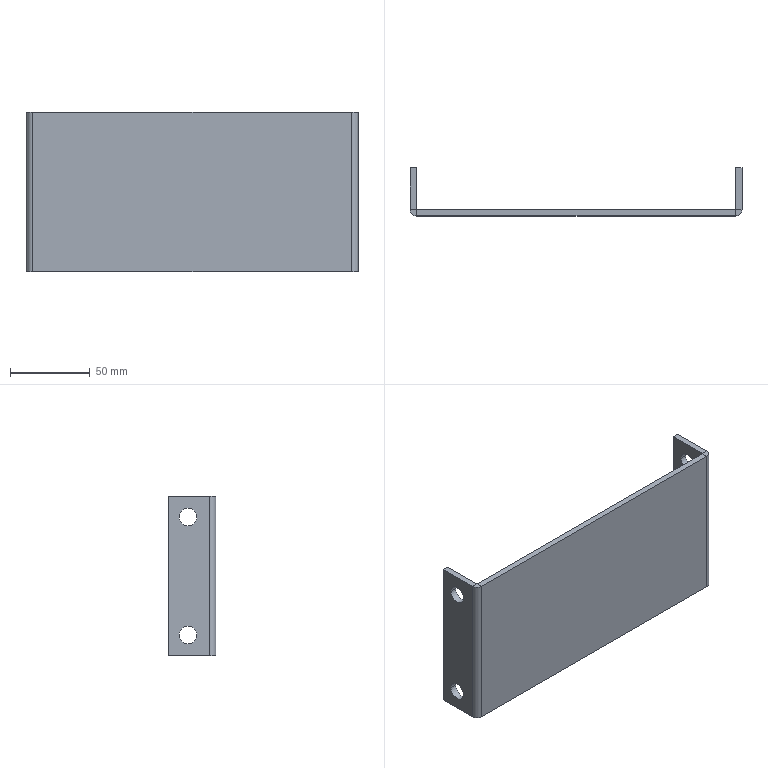Part | SolidWorks | features FlatPattern 1, ICE 1, SMBaseFlange 1, SheetMetal 1 | 1 solid | 30 faces | box 208 x 30 x 100 mm | volume 101724 mm3 | plane 18 | cylinder 12 | commonest cylinder face diameters 11 x8 0.4 x2 8.4 x2
STEP:
#1=CARTESIAN_POINT('',(100.,23.,37.));
#2=VERTEX_POINT('',#1);
#3=CARTESIAN_POINT('',(100.,12.,37.));
#4=VERTEX_POINT('',#3);
#5=CARTESIAN_POINT('',(100.,17.5,37.));
#6=DIRECTION('',(-1.,0.,0.));
#7=DIRECTION('',(0.,-1.,0.));
#8=AXIS2_PLACEMENT_3D('',#5,#6,#7);
#9=CIRCLE('',#8,5.5);
#10=EDGE_CURVE('',#2,#4,#9,.T.);
#11=ORIENTED_EDGE('',*,*,#10,.T.);
#12=CARTESIAN_POINT('',(104.,12.,37.));
#13=VERTEX_POINT('',#12);
#14=CARTESIAN_POINT('',(-104.,12.,37.));
#15=DIRECTION('',(1.,0.,0.));
#16=VECTOR('',#15,1000.);
#17=LINE('',#14,#16);
#18=EDGE_CURVE('',#4,#13,#17,.T.);
#19=ORIENTED_EDGE('',*,*,#18,.T.);
#20=CARTESIAN_POINT('',(104.,23.,37.));
#21=VERTEX_POINT('',#20);
#22=CARTESIAN_POINT('',(104.,17.5,37.));
#23=DIRECTION('',(-1.,0.,0.));
#24=DIRECTION('',(0.,-1.,0.));
#25=AXIS2_PLACEMENT_3D('',#22,#23,#24);
#26=CIRCLE('',#25,5.5);
#27=EDGE_CURVE('',#21,#13,#26,.T.);
#28=ORIENTED_EDGE('',*,*,#27,.F.);
#29=CARTESIAN_POINT('',(-104.,23.,37.));
#30=DIRECTION('',(1.,0.,0.));
#31=VECTOR('',#30,1000.);
#32=LINE('',#29,#31);
#33=EDGE_CURVE('',#2,#21,#32,.T.);
#34=ORIENTED_EDGE('',*,*,#33,.F.);
#35=EDGE_LOOP('',(#11,#19,#28,#34));
#36=FACE_OUTER_BOUND('',#35,.T.);
#37=CARTESIAN_POINT('',(-104.,17.5,37.));
#38=DIRECTION('',(1.,0.,0.));
#39=DIRECTION('',(0.,1.,0.));
#40=AXIS2_PLACEMENT_3D('',#37,#38,#39);
#41=CYLINDRICAL_SURFACE('',#40,5.5);
#42=ADVANCED_FACE('',(#36),#41,.F.);
#43=CARTESIAN_POINT('',(100.,23.,-37.));
#44=VERTEX_POINT('',#43);
#45=CARTESIAN_POINT('',(100.,12.,-37.));
#46=VERTEX_POINT('',#45);
#47=CARTESIAN_POINT('',(100.,17.5,-37.));
#48=DIRECTION('',(-1.,0.,0.));
#49=DIRECTION('',(0.,-1.,0.));
#50=AXIS2_PLACEMENT_3D('',#47,#48,#49);
#51=CIRCLE('',#50,5.5);
#52=EDGE_CURVE('',#44,#46,#51,.T.);
#53=ORIENTED_EDGE('',*,*,#52,.T.);
#54=CARTESIAN_POINT('',(104.,12.,-37.));
#55=VERTEX_POINT('',#54);
#56=CARTESIAN_POINT('',(-104.,12.,-37.));
#57=DIRECTION('',(1.,0.,0.));
#58=VECTOR('',#57,1000.);
#59=LINE('',#56,#58);
#60=EDGE_CURVE('',#46,#55,#59,.T.);
#61=ORIENTED_EDGE('',*,*,#60,.T.);
#62=CARTESIAN_POINT('',(104.,23.,-37.));
#63=VERTEX_POINT('',#62);
#64=CARTESIAN_POINT('',(104.,17.5,-37.));
#65=DIRECTION('',(-1.,0.,0.));
#66=DIRECTION('',(0.,-1.,0.));
#67=AXIS2_PLACEMENT_3D('',#64,#65,#66);
#68=CIRCLE('',#67,5.5);
#69=EDGE_CURVE('',#63,#55,#68,.T.);
#70=ORIENTED_EDGE('',*,*,#69,.F.);
#71=CARTESIAN_POINT('',(-104.,23.,-37.));
#72=DIRECTION('',(1.,0.,0.));
#73=VECTOR('',#72,1000.);
#74=LINE('',#71,#73);
#75=EDGE_CURVE('',#44,#63,#74,.T.);
#76=ORIENTED_EDGE('',*,*,#75,.F.);
#77=EDGE_LOOP('',(#53,#61,#70,#76));
#78=FACE_OUTER_BOUND('',#77,.T.);
#79=CARTESIAN_POINT('',(-104.,17.5,-37.));
#80=DIRECTION('',(1.,0.,0.));
#81=DIRECTION('',(0.,1.,0.));
#82=AXIS2_PLACEMENT_3D('',#79,#80,#81);
#83=CYLINDRICAL_SURFACE('',#82,5.5);
#84=ADVANCED_FACE('',(#78),#83,.F.);
#85=CARTESIAN_POINT('',(-104.,12.,37.));
#86=VERTEX_POINT('',#85);
#87=CARTESIAN_POINT('',(-104.,23.,37.));
#88=VERTEX_POINT('',#87);
#89=CARTESIAN_POINT('',(-104.,17.5,37.));
#90=DIRECTION('',(1.,0.,0.));
#91=DIRECTION('',(0.,1.,0.));
#92=AXIS2_PLACEMENT_3D('',#89,#90,#91);
#93=CIRCLE('',#92,5.5);
#94=EDGE_CURVE('',#86,#88,#93,.T.);
#95=ORIENTED_EDGE('',*,*,#94,.F.);
#96=CARTESIAN_POINT('',(-100.,12.,37.));
#97=VERTEX_POINT('',#96);
#98=CARTESIAN_POINT('',(-104.,12.,37.));
#99=DIRECTION('',(1.,0.,0.));
#100=VECTOR('',#99,1000.);
#101=LINE('',#98,#100);
#102=EDGE_CURVE('',#86,#97,#101,.T.);
#103=ORIENTED_EDGE('',*,*,#102,.T.);
#104=CARTESIAN_POINT('',(-100.,23.,37.));
#105=VERTEX_POINT('',#104);
#106=CARTESIAN_POINT('',(-100.,17.5,37.));
#107=DIRECTION('',(1.,0.,0.));
#108=DIRECTION('',(0.,1.,0.));
#109=AXIS2_PLACEMENT_3D('',#106,#107,#108);
#110=CIRCLE('',#109,5.5);
#111=EDGE_CURVE('',#97,#105,#110,.T.);
#112=ORIENTED_EDGE('',*,*,#111,.T.);
#113=CARTESIAN_POINT('',(-104.,23.,37.));
#114=DIRECTION('',(1.,0.,0.));
#115=VECTOR('',#114,1000.);
#116=LINE('',#113,#115);
#117=EDGE_CURVE('',#88,#105,#116,.T.);
#118=ORIENTED_EDGE('',*,*,#117,.F.);
#119=EDGE_LOOP('',(#95,#103,#112,#118));
#120=FACE_OUTER_BOUND('',#119,.T.);
#121=CARTESIAN_POINT('',(-104.,17.5,37.));
#122=DIRECTION('',(1.,0.,0.));
#123=DIRECTION('',(0.,1.,0.));
#124=AXIS2_PLACEMENT_3D('',#121,#122,#123);
#125=CYLINDRICAL_SURFACE('',#124,5.5);
#126=ADVANCED_FACE('',(#120),#125,.F.);
#127=CARTESIAN_POINT('',(-104.,12.,-37.));
#128=VERTEX_POINT('',#127);
#129=CARTESIAN_POINT('',(-104.,23.,-37.));
#130=VERTEX_POINT('',#129);
#131=CARTESIAN_POINT('',(-104.,17.5,-37.));
#132=DIRECTION('',(1.,0.,0.));
#133=DIRECTION('',(0.,1.,0.));
#134=AXIS2_PLACEMENT_3D('',#131,#132,#133);
#135=CIRCLE('',#134,5.5);
#136=EDGE_CURVE('',#128,#130,#135,.T.);
#137=ORIENTED_EDGE('',*,*,#136,.F.);
#138=CARTESIAN_POINT('',(-100.,12.,-37.));
#139=VERTEX_POINT('',#138);
#140=CARTESIAN_POINT('',(-104.,12.,-37.));
#141=DIRECTION('',(1.,0.,0.));
#142=VECTOR('',#141,1000.);
#143=LINE('',#140,#142);
#144=EDGE_CURVE('',#128,#139,#143,.T.);
#145=ORIENTED_EDGE('',*,*,#144,.T.);
#146=CARTESIAN_POINT('',(-100.,23.,-37.));
#147=VERTEX_POINT('',#146);
#148=CARTESIAN_POINT('',(-100.,17.5,-37.));
#149=DIRECTION('',(1.,0.,0.));
#150=DIRECTION('',(0.,1.,0.));
#151=AXIS2_PLACEMENT_3D('',#148,#149,#150);
#152=CIRCLE('',#151,5.5);
#153=EDGE_CURVE('',#139,#147,#152,.T.);
#154=ORIENTED_EDGE('',*,*,#153,.T.);
#155=CARTESIAN_POINT('',(-104.,23.,-37.));
#156=DIRECTION('',(1.,0.,0.));
#157=VECTOR('',#156,1000.);
#158=LINE('',#155,#157);
#159=EDGE_CURVE('',#130,#147,#158,.T.);
#160=ORIENTED_EDGE('',*,*,#159,.F.);
#161=EDGE_LOOP('',(#137,#145,#154,#160));
#162=FACE_OUTER_BOUND('',#161,.T.);
#163=CARTESIAN_POINT('',(-104.,17.5,-37.));
#164=DIRECTION('',(1.,0.,0.));
#165=DIRECTION('',(0.,1.,0.));
#166=AXIS2_PLACEMENT_3D('',#163,#164,#165);
#167=CYLINDRICAL_SURFACE('',#166,5.5);
#168=ADVANCED_FACE('',(#162),#167,.F.);
#169=CARTESIAN_POINT('',(-104.,4.2,50.));
#170=VERTEX_POINT('',#169);
#171=CARTESIAN_POINT('',(-100.,4.2,50.));
#172=VERTEX_POINT('',#171);
#173=CARTESIAN_POINT('',(-104.,4.2,50.));
#174=DIRECTION('',(1.,0.,0.));
#175=VECTOR('',#174,1000.);
#176=LINE('',#173,#175);
#177=EDGE_CURVE('',#170,#172,#176,.T.);
#178=ORIENTED_EDGE('',*,*,#177,.F.);
#179=CARTESIAN_POINT('',(-99.8,0.,50.));
#180=VERTEX_POINT('',#179);
#181=CARTESIAN_POINT('',(-99.8,4.2,50.));
#182=DIRECTION('',(0.,0.,1.));
#183=DIRECTION('',(-1.,0.,0.));
#184=AXIS2_PLACEMENT_3D('',#181,#182,#183);
#185=CIRCLE('',#184,4.2);
#186=EDGE_CURVE('',#170,#180,#185,.T.);
#187=ORIENTED_EDGE('',*,*,#186,.T.);
#188=CARTESIAN_POINT('',(-99.8,4.,50.));
#189=VERTEX_POINT('',#188);
#190=CARTESIAN_POINT('',(-99.8,4.,50.));
#191=DIRECTION('',(0.,-1.,0.));
#192=VECTOR('',#191,1000.);
#193=LINE('',#190,#192);
#194=EDGE_CURVE('',#189,#180,#193,.T.);
#195=ORIENTED_EDGE('',*,*,#194,.F.);
#196=CARTESIAN_POINT('',(-99.8,4.2,50.));
#197=DIRECTION('',(0.,0.,1.));
#198=DIRECTION('',(1.,0.,0.));
#199=AXIS2_PLACEMENT_3D('',#196,#197,#198);
#200=CIRCLE('',#199,0.2);
#201=EDGE_CURVE('',#172,#189,#200,.T.);
#202=ORIENTED_EDGE('',*,*,#201,.F.);
#203=EDGE_LOOP('',(#178,#187,#195,#202));
#204=FACE_OUTER_BOUND('',#203,.T.);
#205=CARTESIAN_POINT('',(-104.,4.2,50.));
#206=DIRECTION('',(0.,0.,1.));
#207=DIRECTION('',(1.,0.,0.));
#208=AXIS2_PLACEMENT_3D('',#205,#206,#207);
#209=PLANE('',#208);
#210=ADVANCED_FACE('',(#204),#209,.T.);
#211=CARTESIAN_POINT('',(-104.,30.,50.));
#212=VERTEX_POINT('',#211);
#213=CARTESIAN_POINT('',(-104.,30.,50.));
#214=DIRECTION('',(0.,-1.,0.));
#215=VECTOR('',#214,1000.);
#216=LINE('',#213,#215);
#217=EDGE_CURVE('',#212,#170,#216,.T.);
#218=ORIENTED_EDGE('',*,*,#217,.T.);
#219=ORIENTED_EDGE('',*,*,#177,.T.);
#220=CARTESIAN_POINT('',(-100.,30.,50.));
#221=VERTEX_POINT('',#220);
#222=CARTESIAN_POINT('',(-100.,30.,50.));
#223=DIRECTION('',(0.,-1.,0.));
#224=VECTOR('',#223,1000.);
#225=LINE('',#222,#224);
#226=EDGE_CURVE('',#221,#172,#225,.T.);
#227=ORIENTED_EDGE('',*,*,#226,.F.);
#228=CARTESIAN_POINT('',(-104.,30.,50.));
#229=DIRECTION('',(1.,0.,0.));
#230=VECTOR('',#229,1000.);
#231=LINE('',#228,#230);
#232=EDGE_CURVE('',#212,#221,#231,.T.);
#233=ORIENTED_EDGE('',*,*,#232,.F.);
#234=EDGE_LOOP('',(#218,#219,#227,#233));
#235=FACE_OUTER_BOUND('',#234,.T.);
#236=CARTESIAN_POINT('',(-99.8,4.,50.));
#237=DIRECTION('',(0.,0.,1.));
#238=DIRECTION('',(1.,0.,0.));
#239=AXIS2_PLACEMENT_3D('',#236,#237,#238);
#240=PLANE('',#239);
#241=ADVANCED_FACE('',(#235),#240,.T.);
#242=CARTESIAN_POINT('',(-99.8,0.,-50.));
#243=VERTEX_POINT('',#242);
#244=CARTESIAN_POINT('',(-99.8,4.,-50.));
#245=VERTEX_POINT('',#244);
#246=CARTESIAN_POINT('',(-99.8,0.,-50.));
#247=DIRECTION('',(0.,1.,0.));
#248=VECTOR('',#247,1000.);
#249=LINE('',#246,#248);
#250=EDGE_CURVE('',#243,#245,#249,.T.);
#251=ORIENTED_EDGE('',*,*,#250,.F.);
#252=CARTESIAN_POINT('',(-104.,4.2,-50.));
#253=VERTEX_POINT('',#252);
#254=CARTESIAN_POINT('',(-99.8,4.2,-50.));
#255=DIRECTION('',(0.,0.,1.));
#256=DIRECTION('',(-1.,0.,0.));
#257=AXIS2_PLACEMENT_3D('',#254,#255,#256);
#258=CIRCLE('',#257,4.2);
#259=EDGE_CURVE('',#253,#243,#258,.T.);
#260=ORIENTED_EDGE('',*,*,#259,.F.);
#261=CARTESIAN_POINT('',(-100.,4.2,-50.));
#262=VERTEX_POINT('',#261);
#263=CARTESIAN_POINT('',(-100.,4.2,-50.));
#264=DIRECTION('',(-1.,0.,0.));
#265=VECTOR('',#264,1000.);
#266=LINE('',#263,#265);
#267=EDGE_CURVE('',#262,#253,#266,.T.);
#268=ORIENTED_EDGE('',*,*,#267,.F.);
#269=CARTESIAN_POINT('',(-99.8,4.2,-50.));
#270=DIRECTION('',(0.,0.,1.));
#271=DIRECTION('',(1.,0.,0.));
#272=AXIS2_PLACEMENT_3D('',#269,#270,#271);
#273=CIRCLE('',#272,0.2);
#274=EDGE_CURVE('',#262,#245,#273,.T.);
#275=ORIENTED_EDGE('',*,*,#274,.T.);
#276=EDGE_LOOP('',(#251,#260,#268,#275));
#277=FACE_OUTER_BOUND('',#276,.T.);
#278=CARTESIAN_POINT('',(-99.8,0.,-50.));
#279=DIRECTION('',(0.,0.,-1.));
#280=DIRECTION('',(-1.,0.,0.));
#281=AXIS2_PLACEMENT_3D('',#278,#279,#280);
#282=PLANE('',#281);
#283=ADVANCED_FACE('',(#277),#282,.T.);
#284=CARTESIAN_POINT('',(99.8,0.,-50.));
#285=VERTEX_POINT('',#284);
#286=CARTESIAN_POINT('',(-104.,0.,-50.));
#287=DIRECTION('',(1.,0.,0.));
#288=VECTOR('',#287,1000.);
#289=LINE('',#286,#288);
#290=EDGE_CURVE('',#243,#285,#289,.T.);
#291=ORIENTED_EDGE('',*,*,#290,.F.);
#292=ORIENTED_EDGE('',*,*,#250,.T.);
#293=CARTESIAN_POINT('',(99.8,4.,-50.));
#294=VERTEX_POINT('',#293);
#295=CARTESIAN_POINT('',(-104.,4.,-50.));
#296=DIRECTION('',(1.,0.,0.));
#297=VECTOR('',#296,1000.);
#298=LINE('',#295,#297);
#299=EDGE_CURVE('',#245,#294,#298,.T.);
#300=ORIENTED_EDGE('',*,*,#299,.T.);
#301=CARTESIAN_POINT('',(99.8,4.,-50.));
#302=DIRECTION('',(0.,-1.,0.));
#303=VECTOR('',#302,1000.);
#304=LINE('',#301,#303);
#305=EDGE_CURVE('',#294,#285,#304,.T.);
#306=ORIENTED_EDGE('',*,*,#305,.T.);
#307=EDGE_LOOP('',(#291,#292,#300,#306));
#308=FACE_OUTER_BOUND('',#307,.T.);
#309=CARTESIAN_POINT('',(-100.,4.2,-50.));
#310=DIRECTION('',(0.,0.,-1.));
#311=DIRECTION('',(-1.,0.,0.));
#312=AXIS2_PLACEMENT_3D('',#309,#310,#311);
#313=PLANE('',#312);
#314=ADVANCED_FACE('',(#308),#313,.T.);
#315=CARTESIAN_POINT('',(99.8,0.,50.));
#316=VERTEX_POINT('',#315);
#317=CARTESIAN_POINT('',(99.8,4.,50.));
#318=VERTEX_POINT('',#317);
#319=CARTESIAN_POINT('',(99.8,0.,50.));
#320=DIRECTION('',(0.,1.,0.));
#321=VECTOR('',#320,1000.);
#322=LINE('',#319,#321);
#323=EDGE_CURVE('',#316,#318,#322,.T.);
#324=ORIENTED_EDGE('',*,*,#323,.F.);
#325=CARTESIAN_POINT('',(104.,4.2,50.));
#326=VERTEX_POINT('',#325);
#327=CARTESIAN_POINT('',(99.8,4.2,50.));
#328=DIRECTION('',(0.,0.,1.));
#329=DIRECTION('',(-1.,0.,0.));
#330=AXIS2_PLACEMENT_3D('',#327,#328,#329);
#331=CIRCLE('',#330,4.2);
#332=EDGE_CURVE('',#316,#326,#331,.T.);
#333=ORIENTED_EDGE('',*,*,#332,.T.);
#334=CARTESIAN_POINT('',(100.,4.2,50.));
#335=VERTEX_POINT('',#334);
#336=CARTESIAN_POINT('',(100.,4.2,50.));
#337=DIRECTION('',(1.,0.,0.));
#338=VECTOR('',#337,1000.);
#339=LINE('',#336,#338);
#340=EDGE_CURVE('',#335,#326,#339,.T.);
#341=ORIENTED_EDGE('',*,*,#340,.F.);
#342=CARTESIAN_POINT('',(99.8,4.2,50.));
#343=DIRECTION('',(0.,0.,1.));
#344=DIRECTION('',(1.,0.,0.));
#345=AXIS2_PLACEMENT_3D('',#342,#343,#344);
#346=CIRCLE('',#345,0.2);
#347=EDGE_CURVE('',#318,#335,#346,.T.);
#348=ORIENTED_EDGE('',*,*,#347,.F.);
#349=EDGE_LOOP('',(#324,#333,#341,#348));
#350=FACE_OUTER_BOUND('',#349,.T.);
#351=CARTESIAN_POINT('',(99.8,0.,50.));
#352=DIRECTION('',(0.,0.,1.));
#353=DIRECTION('',(1.,0.,0.));
#354=AXIS2_PLACEMENT_3D('',#351,#352,#353);
#355=PLANE('',#354);
#356=ADVANCED_FACE('',(#350),#355,.T.);
#357=CARTESIAN_POINT('',(-104.,0.,50.));
#358=DIRECTION('',(1.,0.,0.));
#359=VECTOR('',#358,1000.);
#360=LINE('',#357,#359);
#361=EDGE_CURVE('',#180,#316,#360,.T.);
#362=ORIENTED_EDGE('',*,*,#361,.T.);
#363=ORIENTED_EDGE('',*,*,#323,.T.);
#364=CARTESIAN_POINT('',(-104.,4.,50.));
#365=DIRECTION('',(1.,0.,0.));
#366=VECTOR('',#365,1000.);
#367=LINE('',#364,#366);
#368=EDGE_CURVE('',#189,#318,#367,.T.);
#369=ORIENTED_EDGE('',*,*,#368,.F.);
#370=ORIENTED_EDGE('',*,*,#194,.T.);
#371=EDGE_LOOP('',(#362,#363,#369,#370));
#372=FACE_OUTER_BOUND('',#371,.T.);
#373=CARTESIAN_POINT('',(100.,4.2,50.));
#374=DIRECTION('',(0.,0.,1.));
#375=DIRECTION('',(1.,0.,0.));
#376=AXIS2_PLACEMENT_3D('',#373,#374,#375);
#377=PLANE('',#376);
#378=ADVANCED_FACE('',(#372),#377,.T.);
#379=CARTESIAN_POINT('',(104.,4.2,-50.));
#380=VERTEX_POINT('',#379);
#381=CARTESIAN_POINT('',(100.,4.2,-50.));
#382=VERTEX_POINT('',#381);
#383=CARTESIAN_POINT('',(104.,4.2,-50.));
#384=DIRECTION('',(-1.,0.,0.));
#385=VECTOR('',#384,1000.);
#386=LINE('',#383,#385);
#387=EDGE_CURVE('',#380,#382,#386,.T.);
#388=ORIENTED_EDGE('',*,*,#387,.F.);
#389=CARTESIAN_POINT('',(99.8,4.2,-50.));
#390=DIRECTION('',(0.,0.,1.));
#391=DIRECTION('',(-1.,0.,0.));
#392=AXIS2_PLACEMENT_3D('',#389,#390,#391);
#393=CIRCLE('',#392,4.2);
#394=EDGE_CURVE('',#285,#380,#393,.T.);
#395=ORIENTED_EDGE('',*,*,#394,.F.);
#396=ORIENTED_EDGE('',*,*,#305,.F.);
#397=CARTESIAN_POINT('',(99.8,4.2,-50.));
#398=DIRECTION('',(0.,0.,1.));
#399=DIRECTION('',(1.,0.,0.));
#400=AXIS2_PLACEMENT_3D('',#397,#398,#399);
#401=CIRCLE('',#400,0.2);
#402=EDGE_CURVE('',#294,#382,#401,.T.);
#403=ORIENTED_EDGE('',*,*,#402,.T.);
#404=EDGE_LOOP('',(#388,#395,#396,#403));
#405=FACE_OUTER_BOUND('',#404,.T.);
#406=CARTESIAN_POINT('',(104.,4.2,-50.));
#407=DIRECTION('',(0.,0.,-1.));
#408=DIRECTION('',(-1.,0.,0.));
#409=AXIS2_PLACEMENT_3D('',#406,#407,#408);
#410=PLANE('',#409);
#411=ADVANCED_FACE('',(#405),#410,.T.);
#412=CARTESIAN_POINT('',(104.,30.,-50.));
#413=VERTEX_POINT('',#412);
#414=CARTESIAN_POINT('',(104.,0.,-50.));
#415=DIRECTION('',(0.,1.,0.));
#416=VECTOR('',#415,1000.);
#417=LINE('',#414,#416);
#418=EDGE_CURVE('',#380,#413,#417,.T.);
#419=ORIENTED_EDGE('',*,*,#418,.F.);
#420=ORIENTED_EDGE('',*,*,#387,.T.);
#421=CARTESIAN_POINT('',(100.,30.,-50.));
#422=VERTEX_POINT('',#421);
#423=CARTESIAN_POINT('',(100.,0.,-50.));
#424=DIRECTION('',(0.,1.,0.));
#425=VECTOR('',#424,1000.);
#426=LINE('',#423,#425);
#427=EDGE_CURVE('',#382,#422,#426,.T.);
#428=ORIENTED_EDGE('',*,*,#427,.T.);
#429=CARTESIAN_POINT('',(100.,30.,-50.));
#430=DIRECTION('',(1.,0.,0.));
#431=VECTOR('',#430,1000.);
#432=LINE('',#429,#431);
#433=EDGE_CURVE('',#422,#413,#432,.T.);
#434=ORIENTED_EDGE('',*,*,#433,.T.);
#435=EDGE_LOOP('',(#419,#420,#428,#434));
#436=FACE_OUTER_BOUND('',#435,.T.);
#437=CARTESIAN_POINT('',(99.8,4.,-50.));
#438=DIRECTION('',(0.,0.,-1.));
#439=DIRECTION('',(-1.,0.,0.));
#440=AXIS2_PLACEMENT_3D('',#437,#438,#439);
#441=PLANE('',#440);
#442=ADVANCED_FACE('',(#436),#441,.T.);
#443=ORIENTED_EDGE('',*,*,#27,.T.);
#444=CARTESIAN_POINT('',(104.,17.5,37.));
#445=DIRECTION('',(-1.,0.,0.));
#446=DIRECTION('',(0.,-1.,0.));
#447=AXIS2_PLACEMENT_3D('',#444,#445,#446);
#448=CIRCLE('',#447,5.5);
#449=EDGE_CURVE('',#13,#21,#448,.T.);
#450=ORIENTED_EDGE('',*,*,#449,.T.);
#451=EDGE_LOOP('',(#443,#450));
#452=FACE_BOUND('',#451,.T.);
#453=ORIENTED_EDGE('',*,*,#69,.T.);
#454=CARTESIAN_POINT('',(104.,17.5,-37.));
#455=DIRECTION('',(-1.,0.,0.));
#456=DIRECTION('',(0.,-1.,0.));
#457=AXIS2_PLACEMENT_3D('',#454,#455,#456);
#458=CIRCLE('',#457,5.5);
#459=EDGE_CURVE('',#55,#63,#458,.T.);
#460=ORIENTED_EDGE('',*,*,#459,.T.);
#461=EDGE_LOOP('',(#453,#460));
#462=FACE_BOUND('',#461,.T.);
#463=ORIENTED_EDGE('',*,*,#418,.T.);
#464=CARTESIAN_POINT('',(104.,30.,50.));
#465=VERTEX_POINT('',#464);
#466=CARTESIAN_POINT('',(104.,30.,50.));
#467=DIRECTION('',(0.,0.,-1.));
#468=VECTOR('',#467,1000.);
#469=LINE('',#466,#468);
#470=EDGE_CURVE('',#465,#413,#469,.T.);
#471=ORIENTED_EDGE('',*,*,#470,.F.);
#472=CARTESIAN_POINT('',(104.,0.,50.));
#473=DIRECTION('',(0.,1.,0.));
#474=VECTOR('',#473,1000.);
#475=LINE('',#472,#474);
#476=EDGE_CURVE('',#326,#465,#475,.T.);
#477=ORIENTED_EDGE('',*,*,#476,.F.);
#478=CARTESIAN_POINT('',(104.,4.2,50.));
#479=DIRECTION('',(0.,0.,-1.));
#480=VECTOR('',#479,1000.);
#481=LINE('',#478,#480);
#482=EDGE_CURVE('',#326,#380,#481,.T.);
#483=ORIENTED_EDGE('',*,*,#482,.T.);
#484=EDGE_LOOP('',(#463,#471,#477,#483));
#485=FACE_OUTER_BOUND('',#484,.T.);
#486=CARTESIAN_POINT('',(104.,0.,50.));
#487=DIRECTION('',(-1.,0.,0.));
#488=DIRECTION('',(0.,-1.,0.));
#489=AXIS2_PLACEMENT_3D('',#486,#487,#488);
#490=PLANE('',#489);
#491=ADVANCED_FACE('',(#452,#462,#485),#490,.F.);
#492=ORIENTED_EDGE('',*,*,#433,.F.);
#493=CARTESIAN_POINT('',(100.,30.,50.));
#494=VERTEX_POINT('',#493);
#495=CARTESIAN_POINT('',(100.,30.,50.));
#496=DIRECTION('',(0.,0.,-1.));
#497=VECTOR('',#496,1000.);
#498=LINE('',#495,#497);
#499=EDGE_CURVE('',#494,#422,#498,.T.);
#500=ORIENTED_EDGE('',*,*,#499,.F.);
#501=CARTESIAN_POINT('',(100.,30.,50.));
#502=DIRECTION('',(1.,0.,0.));
#503=VECTOR('',#502,1000.);
#504=LINE('',#501,#503);
#505=EDGE_CURVE('',#494,#465,#504,.T.);
#506=ORIENTED_EDGE('',*,*,#505,.T.);
#507=ORIENTED_EDGE('',*,*,#470,.T.);
#508=EDGE_LOOP('',(#492,#500,#506,#507));
#509=FACE_OUTER_BOUND('',#508,.T.);
#510=CARTESIAN_POINT('',(100.,30.,50.));
#511=DIRECTION('',(0.,1.,0.));
#512=DIRECTION('',(-1.,0.,0.));
#513=AXIS2_PLACEMENT_3D('',#510,#511,#512);
#514=PLANE('',#513);
#515=ADVANCED_FACE('',(#509),#514,.T.);
#516=ORIENTED_EDGE('',*,*,#10,.F.);
#517=CARTESIAN_POINT('',(100.,17.5,37.));
#518=DIRECTION('',(-1.,0.,0.));
#519=DIRECTION('',(0.,-1.,0.));
#520=AXIS2_PLACEMENT_3D('',#517,#518,#519);
#521=CIRCLE('',#520,5.5);
#522=EDGE_CURVE('',#4,#2,#521,.T.);
#523=ORIENTED_EDGE('',*,*,#522,.F.);
#524=EDGE_LOOP('',(#516,#523));
#525=FACE_BOUND('',#524,.T.);
#526=ORIENTED_EDGE('',*,*,#52,.F.);
#527=CARTESIAN_POINT('',(100.,17.5,-37.));
#528=DIRECTION('',(-1.,0.,0.));
#529=DIRECTION('',(0.,-1.,0.));
#530=AXIS2_PLACEMENT_3D('',#527,#528,#529);
#531=CIRCLE('',#530,5.5);
#532=EDGE_CURVE('',#46,#44,#531,.T.);
#533=ORIENTED_EDGE('',*,*,#532,.F.);
#534=EDGE_LOOP('',(#526,#533));
#535=FACE_BOUND('',#534,.T.);
#536=ORIENTED_EDGE('',*,*,#427,.F.);
#537=CARTESIAN_POINT('',(100.,4.2,50.));
#538=DIRECTION('',(0.,0.,-1.));
#539=VECTOR('',#538,1000.);
#540=LINE('',#537,#539);
#541=EDGE_CURVE('',#335,#382,#540,.T.);
#542=ORIENTED_EDGE('',*,*,#541,.F.);
#543=CARTESIAN_POINT('',(100.,0.,50.));
#544=DIRECTION('',(0.,1.,0.));
#545=VECTOR('',#544,1000.);
#546=LINE('',#543,#545);
#547=EDGE_CURVE('',#335,#494,#546,.T.);
#548=ORIENTED_EDGE('',*,*,#547,.T.);
#549=ORIENTED_EDGE('',*,*,#499,.T.);
#550=EDGE_LOOP('',(#536,#542,#548,#549));
#551=FACE_OUTER_BOUND('',#550,.T.);
#552=CARTESIAN_POINT('',(100.,0.,50.));
#553=DIRECTION('',(-1.,0.,0.));
#554=DIRECTION('',(0.,-1.,0.));
#555=AXIS2_PLACEMENT_3D('',#552,#553,#554);
#556=PLANE('',#555);
#557=ADVANCED_FACE('',(#525,#535,#551),#556,.T.);
#558=ORIENTED_EDGE('',*,*,#402,.F.);
#559=CARTESIAN_POINT('',(99.8,4.,50.));
#560=DIRECTION('',(0.,0.,-1.));
#561=VECTOR('',#560,1000.);
#562=LINE('',#559,#561);
#563=EDGE_CURVE('',#318,#294,#562,.T.);
#564=ORIENTED_EDGE('',*,*,#563,.F.);
#565=ORIENTED_EDGE('',*,*,#347,.T.);
#566=ORIENTED_EDGE('',*,*,#541,.T.);
#567=EDGE_LOOP('',(#558,#564,#565,#566));
#568=FACE_OUTER_BOUND('',#567,.T.);
#569=CARTESIAN_POINT('',(99.8,4.2,50.));
#570=DIRECTION('',(0.,0.,-1.));
#571=DIRECTION('',(-1.,0.,0.));
#572=AXIS2_PLACEMENT_3D('',#569,#570,#571);
#573=CYLINDRICAL_SURFACE('',#572,0.2);
#574=ADVANCED_FACE('',(#568),#573,.F.);
#575=ORIENTED_EDGE('',*,*,#299,.F.);
#576=CARTESIAN_POINT('',(-99.8,4.,50.));
#577=DIRECTION('',(0.,0.,-1.));
#578=VECTOR('',#577,1000.);
#579=LINE('',#576,#578);
#580=EDGE_CURVE('',#189,#245,#579,.T.);
#581=ORIENTED_EDGE('',*,*,#580,.F.);
#582=ORIENTED_EDGE('',*,*,#368,.T.);
#583=ORIENTED_EDGE('',*,*,#563,.T.);
#584=EDGE_LOOP('',(#575,#581,#582,#583));
#585=FACE_OUTER_BOUND('',#584,.T.);
#586=CARTESIAN_POINT('',(-104.,4.,50.));
#587=DIRECTION('',(0.,1.,0.));
#588=DIRECTION('',(0.,0.,1.));
#589=AXIS2_PLACEMENT_3D('',#586,#587,#588);
#590=PLANE('',#589);
#591=ADVANCED_FACE('',(#585),#590,.T.);
#592=ORIENTED_EDGE('',*,*,#274,.F.);
#593=CARTESIAN_POINT('',(-100.,4.2,50.));
#594=DIRECTION('',(0.,0.,-1.));
#595=VECTOR('',#594,1000.);
#596=LINE('',#593,#595);
#597=EDGE_CURVE('',#172,#262,#596,.T.);
#598=ORIENTED_EDGE('',*,*,#597,.F.);
#599=ORIENTED_EDGE('',*,*,#201,.T.);
#600=ORIENTED_EDGE('',*,*,#580,.T.);
#601=EDGE_LOOP('',(#592,#598,#599,#600));
#602=FACE_OUTER_BOUND('',#601,.T.);
#603=CARTESIAN_POINT('',(-99.8,4.2,50.));
#604=DIRECTION('',(0.,0.,-1.));
#605=DIRECTION('',(-1.,0.,0.));
#606=AXIS2_PLACEMENT_3D('',#603,#604,#605);
#607=CYLINDRICAL_SURFACE('',#606,0.2);
#608=ADVANCED_FACE('',(#602),#607,.F.);
#609=CARTESIAN_POINT('',(-100.,17.5,37.));
#610=DIRECTION('',(1.,0.,0.));
#611=DIRECTION('',(0.,1.,0.));
#612=AXIS2_PLACEMENT_3D('',#609,#610,#611);
#613=CIRCLE('',#612,5.5);
#614=EDGE_CURVE('',#105,#97,#613,.T.);
#615=ORIENTED_EDGE('',*,*,#614,.F.);
#616=ORIENTED_EDGE('',*,*,#111,.F.);
#617=EDGE_LOOP('',(#615,#616));
#618=FACE_BOUND('',#617,.T.);
#619=CARTESIAN_POINT('',(-100.,17.5,-37.));
#620=DIRECTION('',(1.,0.,0.));
#621=DIRECTION('',(0.,1.,0.));
#622=AXIS2_PLACEMENT_3D('',#619,#620,#621);
#623=CIRCLE('',#622,5.5);
#624=EDGE_CURVE('',#147,#139,#623,.T.);
#625=ORIENTED_EDGE('',*,*,#624,.F.);
#626=ORIENTED_EDGE('',*,*,#153,.F.);
#627=EDGE_LOOP('',(#625,#626));
#628=FACE_BOUND('',#627,.T.);
#629=CARTESIAN_POINT('',(-100.,30.,-50.));
#630=VERTEX_POINT('',#629);
#631=CARTESIAN_POINT('',(-100.,30.,-50.));
#632=DIRECTION('',(0.,-1.,0.));
#633=VECTOR('',#632,1000.);
#634=LINE('',#631,#633);
#635=EDGE_CURVE('',#630,#262,#634,.T.);
#636=ORIENTED_EDGE('',*,*,#635,.F.);
#637=CARTESIAN_POINT('',(-100.,30.,50.));
#638=DIRECTION('',(0.,0.,-1.));
#639=VECTOR('',#638,1000.);
#640=LINE('',#637,#639);
#641=EDGE_CURVE('',#221,#630,#640,.T.);
#642=ORIENTED_EDGE('',*,*,#641,.F.);
#643=ORIENTED_EDGE('',*,*,#226,.T.);
#644=ORIENTED_EDGE('',*,*,#597,.T.);
#645=EDGE_LOOP('',(#636,#642,#643,#644));
#646=FACE_OUTER_BOUND('',#645,.T.);
#647=CARTESIAN_POINT('',(-100.,30.,50.));
#648=DIRECTION('',(1.,0.,0.));
#649=DIRECTION('',(0.,1.,0.));
#650=AXIS2_PLACEMENT_3D('',#647,#648,#649);
#651=PLANE('',#650);
#652=ADVANCED_FACE('',(#618,#628,#646),#651,.T.);
#653=CARTESIAN_POINT('',(-104.,30.,-50.));
#654=VERTEX_POINT('',#653);
#655=CARTESIAN_POINT('',(-104.,30.,-50.));
#656=DIRECTION('',(1.,0.,0.));
#657=VECTOR('',#656,1000.);
#658=LINE('',#655,#657);
#659=EDGE_CURVE('',#654,#630,#658,.T.);
#660=ORIENTED_EDGE('',*,*,#659,.F.);
#661=CARTESIAN_POINT('',(-104.,30.,50.));
#662=DIRECTION('',(0.,0.,-1.));
#663=VECTOR('',#662,1000.);
#664=LINE('',#661,#663);
#665=EDGE_CURVE('',#212,#654,#664,.T.);
#666=ORIENTED_EDGE('',*,*,#665,.F.);
#667=ORIENTED_EDGE('',*,*,#232,.T.);
#668=ORIENTED_EDGE('',*,*,#641,.T.);
#669=EDGE_LOOP('',(#660,#666,#667,#668));
#670=FACE_OUTER_BOUND('',#669,.T.);
#671=CARTESIAN_POINT('',(-104.,30.,50.));
#672=DIRECTION('',(0.,1.,0.));
#673=DIRECTION('',(-1.,0.,0.));
#674=AXIS2_PLACEMENT_3D('',#671,#672,#673);
#675=PLANE('',#674);
#676=ADVANCED_FACE('',(#670),#675,.T.);
#677=CARTESIAN_POINT('',(-104.,17.5,37.));
#678=DIRECTION('',(1.,0.,0.));
#679=DIRECTION('',(0.,1.,0.));
#680=AXIS2_PLACEMENT_3D('',#677,#678,#679);
#681=CIRCLE('',#680,5.5);
#682=EDGE_CURVE('',#88,#86,#681,.T.);
#683=ORIENTED_EDGE('',*,*,#682,.T.);
#684=ORIENTED_EDGE('',*,*,#94,.T.);
#685=EDGE_LOOP('',(#683,#684));
#686=FACE_BOUND('',#685,.T.);
#687=CARTESIAN_POINT('',(-104.,17.5,-37.));
#688=DIRECTION('',(1.,0.,0.));
#689=DIRECTION('',(0.,1.,0.));
#690=AXIS2_PLACEMENT_3D('',#687,#688,#689);
#691=CIRCLE('',#690,5.5);
#692=EDGE_CURVE('',#130,#128,#691,.T.);
#693=ORIENTED_EDGE('',*,*,#692,.T.);
#694=ORIENTED_EDGE('',*,*,#136,.T.);
#695=EDGE_LOOP('',(#693,#694));
#696=FACE_BOUND('',#695,.T.);
#697=CARTESIAN_POINT('',(-104.,30.,-50.));
#698=DIRECTION('',(0.,-1.,0.));
#699=VECTOR('',#698,1000.);
#700=LINE('',#697,#699);
#701=EDGE_CURVE('',#654,#253,#700,.T.);
#702=ORIENTED_EDGE('',*,*,#701,.T.);
#703=CARTESIAN_POINT('',(-104.,4.2,50.));
#704=DIRECTION('',(0.,0.,-1.));
#705=VECTOR('',#704,1000.);
#706=LINE('',#703,#705);
#707=EDGE_CURVE('',#170,#253,#706,.T.);
#708=ORIENTED_EDGE('',*,*,#707,.F.);
#709=ORIENTED_EDGE('',*,*,#217,.F.);
#710=ORIENTED_EDGE('',*,*,#665,.T.);
#711=EDGE_LOOP('',(#702,#708,#709,#710));
#712=FACE_OUTER_BOUND('',#711,.T.);
#713=CARTESIAN_POINT('',(-104.,30.,50.));
#714=DIRECTION('',(1.,0.,0.));
#715=DIRECTION('',(0.,1.,0.));
#716=AXIS2_PLACEMENT_3D('',#713,#714,#715);
#717=PLANE('',#716);
#718=ADVANCED_FACE('',(#686,#696,#712),#717,.F.);
#719=ORIENTED_EDGE('',*,*,#259,.T.);
#720=CARTESIAN_POINT('',(-99.8,0.,50.));
#721=DIRECTION('',(0.,0.,-1.));
#722=VECTOR('',#721,1000.);
#723=LINE('',#720,#722);
#724=EDGE_CURVE('',#180,#243,#723,.T.);
#725=ORIENTED_EDGE('',*,*,#724,.F.);
#726=ORIENTED_EDGE('',*,*,#186,.F.);
#727=ORIENTED_EDGE('',*,*,#707,.T.);
#728=EDGE_LOOP('',(#719,#725,#726,#727));
#729=FACE_OUTER_BOUND('',#728,.T.);
#730=CARTESIAN_POINT('',(-99.8,4.2,50.));
#731=DIRECTION('',(0.,0.,-1.));
#732=DIRECTION('',(-1.,0.,0.));
#733=AXIS2_PLACEMENT_3D('',#730,#731,#732);
#734=CYLINDRICAL_SURFACE('',#733,4.2);
#735=ADVANCED_FACE('',(#729),#734,.T.);
#736=ORIENTED_EDGE('',*,*,#290,.T.);
#737=CARTESIAN_POINT('',(99.8,0.,50.));
#738=DIRECTION('',(0.,0.,-1.));
#739=VECTOR('',#738,1000.);
#740=LINE('',#737,#739);
#741=EDGE_CURVE('',#316,#285,#740,.T.);
#742=ORIENTED_EDGE('',*,*,#741,.F.);
#743=ORIENTED_EDGE('',*,*,#361,.F.);
#744=ORIENTED_EDGE('',*,*,#724,.T.);
#745=EDGE_LOOP('',(#736,#742,#743,#744));
#746=FACE_OUTER_BOUND('',#745,.T.);
#747=CARTESIAN_POINT('',(-104.,0.,50.));
#748=DIRECTION('',(0.,1.,0.));
#749=DIRECTION('',(0.,0.,1.));
#750=AXIS2_PLACEMENT_3D('',#747,#748,#749);
#751=PLANE('',#750);
#752=ADVANCED_FACE('',(#746),#751,.F.);
#753=ORIENTED_EDGE('',*,*,#394,.T.);
#754=ORIENTED_EDGE('',*,*,#482,.F.);
#755=ORIENTED_EDGE('',*,*,#332,.F.);
#756=ORIENTED_EDGE('',*,*,#741,.T.);
#757=EDGE_LOOP('',(#753,#754,#755,#756));
#758=FACE_OUTER_BOUND('',#757,.T.);
#759=CARTESIAN_POINT('',(99.8,4.2,50.));
#760=DIRECTION('',(0.,0.,-1.));
#761=DIRECTION('',(-1.,0.,0.));
#762=AXIS2_PLACEMENT_3D('',#759,#760,#761);
#763=CYLINDRICAL_SURFACE('',#762,4.2);
#764=ADVANCED_FACE('',(#758),#763,.T.);
#765=ORIENTED_EDGE('',*,*,#476,.T.);
#766=ORIENTED_EDGE('',*,*,#505,.F.);
#767=ORIENTED_EDGE('',*,*,#547,.F.);
#768=ORIENTED_EDGE('',*,*,#340,.T.);
#769=EDGE_LOOP('',(#765,#766,#767,#768));
#770=FACE_OUTER_BOUND('',#769,.T.);
#771=CARTESIAN_POINT('',(99.8,4.2,50.));
#772=DIRECTION('',(0.,0.,1.));
#773=DIRECTION('',(1.,0.,0.));
#774=AXIS2_PLACEMENT_3D('',#771,#772,#773);
#775=PLANE('',#774);
#776=ADVANCED_FACE('',(#770),#775,.T.);
#777=ORIENTED_EDGE('',*,*,#635,.T.);
#778=ORIENTED_EDGE('',*,*,#267,.T.);
#779=ORIENTED_EDGE('',*,*,#701,.F.);
#780=ORIENTED_EDGE('',*,*,#659,.T.);
#781=EDGE_LOOP('',(#777,#778,#779,#780));
#782=FACE_OUTER_BOUND('',#781,.T.);
#783=CARTESIAN_POINT('',(99.8,4.2,-50.));
#784=DIRECTION('',(0.,0.,1.));
#785=DIRECTION('',(1.,0.,0.));
#786=AXIS2_PLACEMENT_3D('',#783,#784,#785);
#787=PLANE('',#786);
#788=ADVANCED_FACE('',(#782),#787,.F.);
#789=ORIENTED_EDGE('',*,*,#144,.F.);
#790=ORIENTED_EDGE('',*,*,#692,.F.);
#791=ORIENTED_EDGE('',*,*,#159,.T.);
#792=ORIENTED_EDGE('',*,*,#624,.T.);
#793=EDGE_LOOP('',(#789,#790,#791,#792));
#794=FACE_OUTER_BOUND('',#793,.T.);
#795=CARTESIAN_POINT('',(-104.,17.5,-37.));
#796=DIRECTION('',(1.,0.,0.));
#797=DIRECTION('',(0.,1.,0.));
#798=AXIS2_PLACEMENT_3D('',#795,#796,#797);
#799=CYLINDRICAL_SURFACE('',#798,5.5);
#800=ADVANCED_FACE('',(#794),#799,.F.);
#801=ORIENTED_EDGE('',*,*,#102,.F.);
#802=ORIENTED_EDGE('',*,*,#682,.F.);
#803=ORIENTED_EDGE('',*,*,#117,.T.);
#804=ORIENTED_EDGE('',*,*,#614,.T.);
#805=EDGE_LOOP('',(#801,#802,#803,#804));
#806=FACE_OUTER_BOUND('',#805,.T.);
#807=CARTESIAN_POINT('',(-104.,17.5,37.));
#808=DIRECTION('',(1.,0.,0.));
#809=DIRECTION('',(0.,1.,0.));
#810=AXIS2_PLACEMENT_3D('',#807,#808,#809);
#811=CYLINDRICAL_SURFACE('',#810,5.5);
#812=ADVANCED_FACE('',(#806),#811,.F.);
#813=ORIENTED_EDGE('',*,*,#60,.F.);
#814=ORIENTED_EDGE('',*,*,#532,.T.);
#815=ORIENTED_EDGE('',*,*,#75,.T.);
#816=ORIENTED_EDGE('',*,*,#459,.F.);
#817=EDGE_LOOP('',(#813,#814,#815,#816));
#818=FACE_OUTER_BOUND('',#817,.T.);
#819=CARTESIAN_POINT('',(-104.,17.5,-37.));
#820=DIRECTION('',(1.,0.,0.));
#821=DIRECTION('',(0.,1.,0.));
#822=AXIS2_PLACEMENT_3D('',#819,#820,#821);
#823=CYLINDRICAL_SURFACE('',#822,5.5);
#824=ADVANCED_FACE('',(#818),#823,.F.);
#825=ORIENTED_EDGE('',*,*,#18,.F.);
#826=ORIENTED_EDGE('',*,*,#522,.T.);
#827=ORIENTED_EDGE('',*,*,#33,.T.);
#828=ORIENTED_EDGE('',*,*,#449,.F.);
#829=EDGE_LOOP('',(#825,#826,#827,#828));
#830=FACE_OUTER_BOUND('',#829,.T.);
#831=CARTESIAN_POINT('',(-104.,17.5,37.));
#832=DIRECTION('',(1.,0.,0.));
#833=DIRECTION('',(0.,1.,0.));
#834=AXIS2_PLACEMENT_3D('',#831,#832,#833);
#835=CYLINDRICAL_SURFACE('',#834,5.5);
#836=ADVANCED_FACE('',(#830),#835,.F.);
#837=CLOSED_SHELL('',(#42,#84,#126,#168,#210,#241,#283,#314,#356,#378,#411,#442,#491,#515,#557,#574,#591,#608,#652,#676,#718,#735,#752,#764,#776,#788,#800,#812,#824,#836));
#838=MANIFOLD_SOLID_BREP('',#837);
#839=CARTESIAN_POINT('',(0.,0.,0.));
#840=DIRECTION('',(0.,0.,1.));
#841=DIRECTION('',(1.,0.,0.));
#842=AXIS2_PLACEMENT_3D('',#839,#840,#841);
#843=(LENGTH_UNIT()NAMED_UNIT(*)SI_UNIT(.MILLI.,.METRE.));
#844=UNCERTAINTY_MEASURE_WITH_UNIT(LENGTH_MEASURE(0.00001),#843,'','');
#845=(NAMED_UNIT(*)PLANE_ANGLE_UNIT()SI_UNIT($,.RADIAN.));
#846=(NAMED_UNIT(*)SI_UNIT($,.STERADIAN.)SOLID_ANGLE_UNIT());
#847=(GEOMETRIC_REPRESENTATION_CONTEXT(3)GLOBAL_UNCERTAINTY_ASSIGNED_CONTEXT((#844))GLOBAL_UNIT_ASSIGNED_CONTEXT((#843,#845,#846))REPRESENTATION_CONTEXT('',''));
#848=ADVANCED_BREP_SHAPE_REPRESENTATION('',(#838,#842),#847);